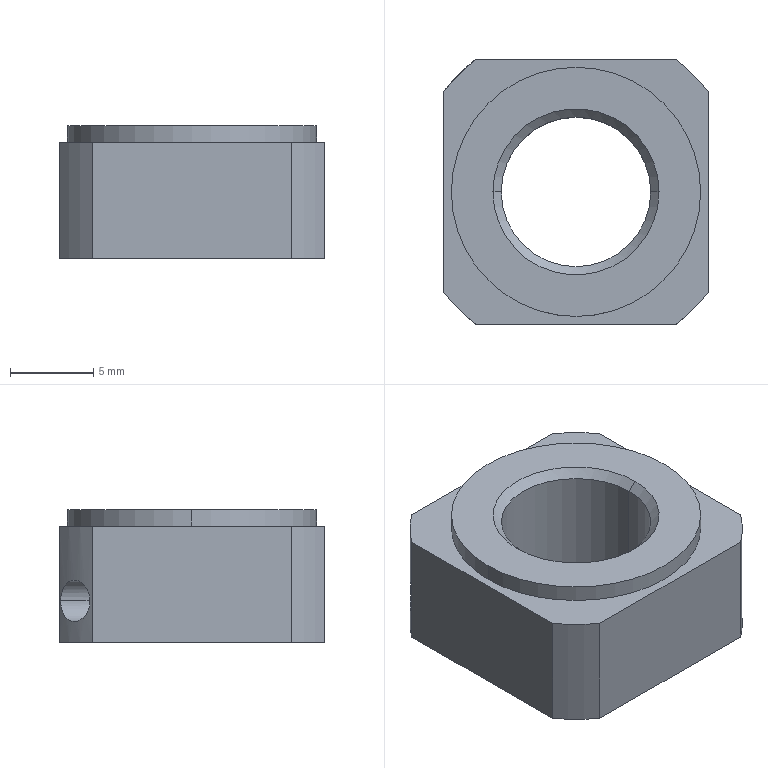Part | STEP file | 1 solid | 21 faces | box 16 x 16 x 8 mm | volume 1375 mm3 | cylinder 10 | plane 7 | cone 4 | commonest cylinder face diameters 20 x4 2.5 x2 9 x2 15 x2